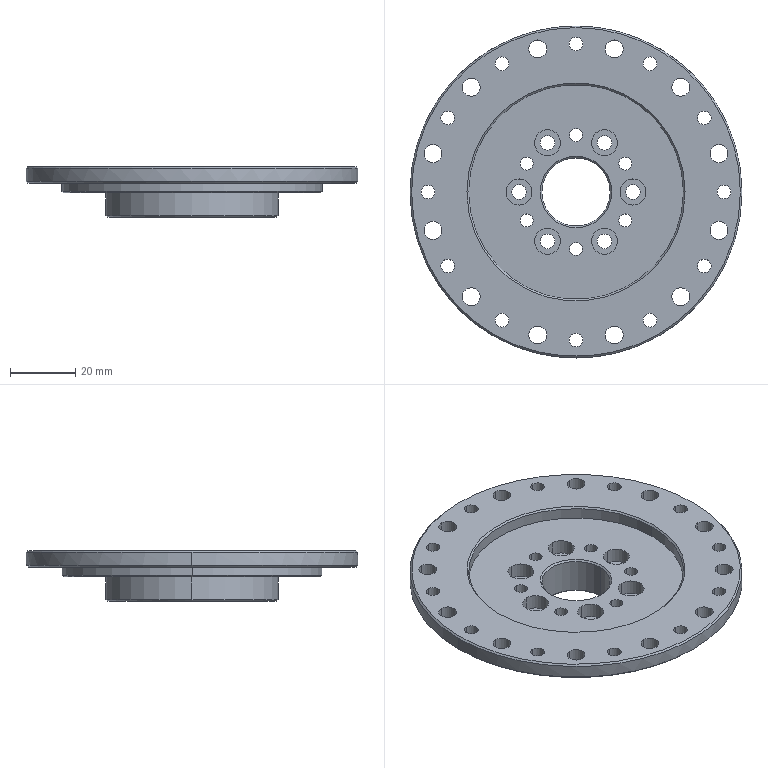CAM job | NX | 3-axis milling, drilling | part box 102 x 102 x 15.5 mm | stock box 112 x 112 x 26.5 mm
Tools:
number,name,description,diameter,corner_radius,flute_length,length,flutes
19,D80,Milling Tool-5 Parameters,80.0,0.0,50.0,75.0,2
15,D10,Milling Tool-5 Parameters,10.0,0.0,50.0,75.0,2
14,D10JING,Milling Tool-5 Parameters,10.0,0.0,50.0,75.0,2
1,D6A45,Milling Tool-5 Parameters,6.0,0.0,50.0,75.0,2
4,4.2ZT,Drilling Tool,4.2,0.0,35.0,50.0,2
9,5.5ZT,Drilling Tool,5.5,0.0,35.0,50.0,2
8,4.5ZT,Drilling Tool,4.5,0.0,35.0,50.0,2
7,3.5ZT,Drilling Tool,3.5,0.0,35.0,50.0,2
12,D6,Milling Tool-5 Parameters,6.0,0.0,50.0,75.0,2
16,D3,Milling Tool-5 Parameters,3.0,0.0,50.0,75.0,2
Operations:
program,operation,operation_type,tool,method,geometry_group,spindle_rpm,surface_speed,feed_per_tooth,feed_cut,feed_plunge,cut_length_mm,path_length_mm,cut_time_min,machine_time_min
1,FLOOR_WALL_COPY,VolumeBased25DMillingOperation,D80,METHOD,A,6500.0,1633.0,0.1154,1500.0,100.0,632.621,686.621,0.4217,0.4271
1,ADAPTIVE_MILLING,CavityMilling,D10,METHOD,A,9500.0,298.0,0.1579,3000.0,1000.0,7394.92,7732.664,3.178,3.211
1,ZLEVEL_PROFILE_COPY_1_COPY_COPY_1,ZLevelMilling,D10JING,METHOD,A,9500.0,298.0,0.0632,1200.0,1000.0,359.358,448.358,0.3001,0.309
1,ZLEVEL_PROFILE_COPY_1_COPY_COPY_1_COPY,ZLevelMilling,D10JING,METHOD,A,9500.0,298.0,0.0632,1200.0,1000.0,43.848,132.848,0.0373,0.0462
1,FLOOR_WALL_COPY_1_COPY,VolumeBased25DMillingOperation,D10JING,METHOD,A,9500.0,298.0,0.0632,1200.0,1000.0,769.62,831.62,0.6429,0.6491
1,DRILLING_COPY_1,Operation,D6A45,METHOD,A,5000.0,94.0,0.035,350.0,0.0,148.0,897.604,0.4229,0.4978
1,DRILLING_COPY_COPY_COPY_2_COPY,Operation,4.2ZT,METHOD,A,2000.0,20.0,0.045,180.0,0.0,129.142,612.455,0.7175,0.7658
1,DRILLING_COPY_COPY_COPY_2_COPY_COPY,Operation,5.5ZT,METHOD,A,2000.0,20.0,0.045,180.0,0.0,133.828,621.828,0.7435,0.7923
1,DRILLING_COPY_COPY_COPY_2,Operation,4.5ZT,METHOD,A,2000.0,20.0,0.045,180.0,0.0,104.112,380,0.5784,0.606
1,DRILLING_COPY_COPY_COPY_2_COPY_1,Operation,3.5ZT,METHOD,A,2000.0,20.0,0.045,180.0,0.0,102.309,376.394,0.5684,0.5958
1,HOLE_MILLING,CylinderMilling,D6,METHOD,A,9500.0,179.0,0.0737,1400.0,100.0,538.185,1058.285,0.3844,0.4364
1,HOLE_MILLING_COPY,CylinderMilling,D3,METHOD,A,9500.0,89.0,0.0632,1200.0,100.0,692.281,1253.781,0.5769,0.6331
1,PLANAR_MILL_COPY_COPY_COPY_COPY_COPY_COPY_1,PlanarMilling,D6A45,METHOD,A,9500.0,179.0,0.0658,1250.0,100.0,971.014,2963.646,0.7768,0.9761
1,PLANAR_MILL_COPY_COPY_COPY_COPY_COPY_COPY_1_COPY,PlanarMilling,D6A45,METHOD,A,9500.0,179.0,0.0658,1250.0,100.0,299.844,1290.649,0.2399,0.339
1,CUTTERCOMP14,ZLevelMilling,D10JING,METHOD,A,9500.0,298.0,0.0632,1200.0,1000.0,183.513,249.513,0.1536,0.1602
1,CUTTERCOMP16,CylinderMilling,D3,METHOD,A,9500.0,89.0,0.0526,1000.0,100.0,241.289,802.789,0.2413,0.2974
2,FLOOR_WALL_COPY_COPY,VolumeBased25DMillingOperation,D80,METHOD,B,6500.0,1633.0,0.1154,1500.0,100.0,5983.809,8134.559,3.989,4.204
2,ADAPTIVE_MILLING_COPY,CavityMilling,D10,METHOD,B,9500.0,298.0,0.1579,3000.0,1000.0,7948.917,8167.226,2.656,2.678
2,FLOOR_WALL_COPY_1_COPY_COPY,VolumeBased25DMillingOperation,D10JING,METHOD,B,9500.0,298.0,0.0632,1200.0,1000.0,2137.599,2306.2,1.786,1.803
2,PLANAR_MILL_COPY_COPY_COPY_COPY_COPY_COPY_1_COPY_1,PlanarMilling,D6A45,METHOD,B,9500.0,179.0,0.0658,1250.0,100.0,241.41,378.81,0.1931,0.2069
2,PLANAR_MILL_COPY_COPY_COPY_COPY_COPY_COPY_1_COPY_1_COPY,PlanarMilling,D6A45,METHOD,B,9500.0,179.0,0.0658,1250.0,100.0,260.82,335.22,0.2087,0.2161
2,PLANAR_MILL_COPY_COPY_COPY_COPY_COPY_COPY_1_COPY_1_COPY_COPY,PlanarMilling,D6A45,METHOD,B,9500.0,179.0,0.0658,1250.0,100.0,329.935,410.335,0.2639,0.272